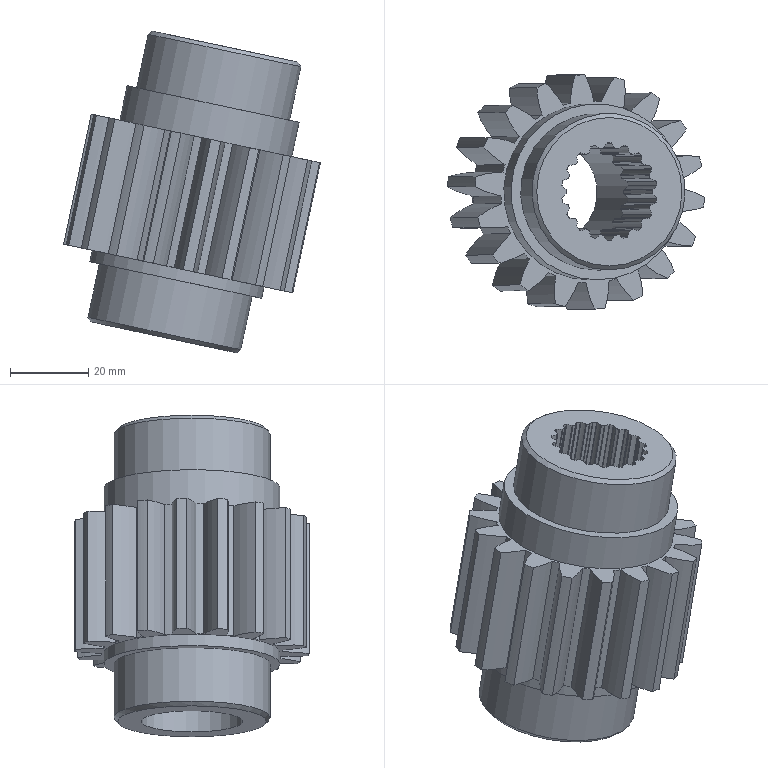Part | STEP file | HL4GZ-1.862.551 (cutter mechanism pinion shaft) | 1 solid | 230 faces | box 65.702 x 59.943 x 82.24 mm | volume 96553 mm3 | cylinder 221 | plane 7 | cone 2 | commonest cylinder face diameters 0.4 x72 9.119 x36 47.047 x36 22.5 x18 25 x18 46.5 x18